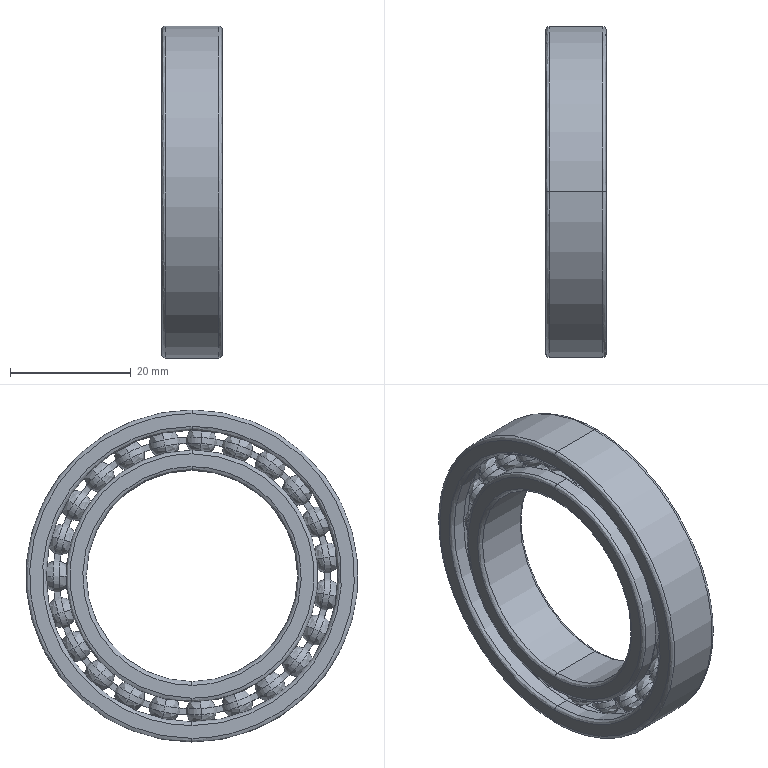Part | SolidWorks | features BaseBody 25 | 25 solids | 269 faces | box 10 x 55 x 55 mm | volume 10471 mm3 | spline 117 | cylinder 102 | plane 50 | commonest cylinder face diameters 44 x45 46 x45 41.667 x4 48.333 x4 35 x2 55 x2